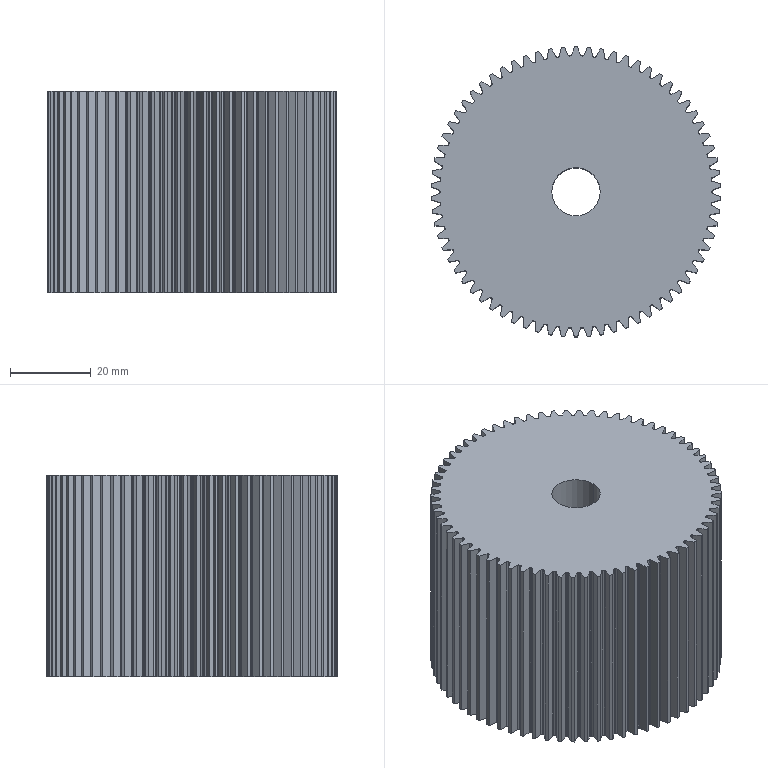Part | SolidWorks | features ICE 2, BaseBody 1 | 1 solid | 455 faces | box 71.959 x 72 x 50 mm | volume 185483 mm3 | cylinder 313 | plane 142 | commonest cylinder face diameters 0.5 x170 67.5 x71 72 x70 12 x2